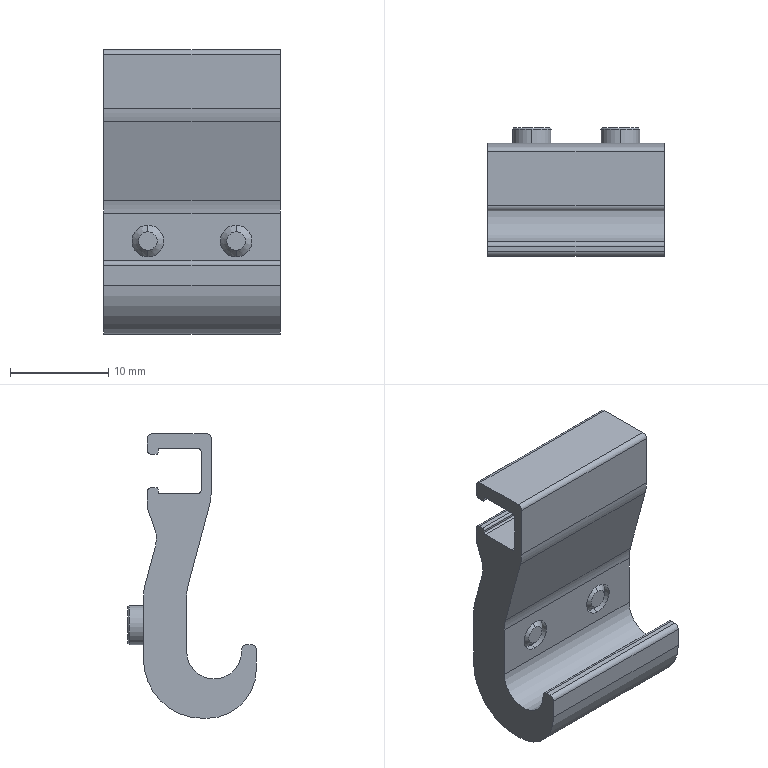Part | SolidWorks | features BaseBody 1 | 1 solid | 75 faces | box 18 x 13.1 x 29 mm | volume 2646 mm3 | plane 40 | cylinder 27 | cone 8 | commonest cylinder face diameters 0.4 x4 0.8 x4 1 x4 3.242 x4 4 x4 10 x4